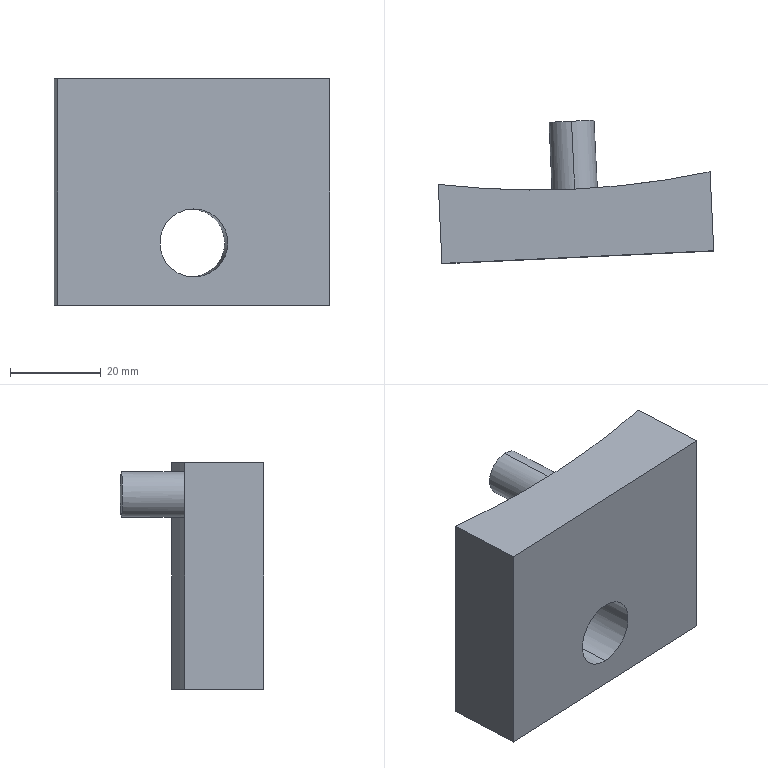Part | SolidWorks | features BaseBody 1 | 1 solid | 11 faces | box 60.748 x 31.599 x 50 mm | volume 45964 mm3 | plane 6 | cylinder 5 | commonest cylinder face diameters 10 x2 15 x2 370 x1
STEP:
#1=CARTESIAN_POINT('',(272.068,803.412,-350.888));
#2=VERTEX_POINT('',#1);
#3=CARTESIAN_POINT('',(272.068,803.412,-365.888));
#4=VERTEX_POINT('',#3);
#5=CARTESIAN_POINT('',(272.068,803.412,-358.388));
#6=DIRECTION('',(-0.04661,0.9989,0.));
#7=DIRECTION('',(0.,0.,1.));
#8=AXIS2_PLACEMENT_3D('',#5,#6,#7);
#9=CIRCLE('',#8,7.5);
#10=EDGE_CURVE('',#2,#4,#9,.T.);
#11=ORIENTED_EDGE('',*,*,#10,.T.);
#12=CARTESIAN_POINT('',(272.068,803.412,-358.388));
#13=DIRECTION('',(-0.04661,0.9989,0.));
#14=DIRECTION('',(0.,0.,1.));
#15=AXIS2_PLACEMENT_3D('',#12,#13,#14);
#16=CIRCLE('',#15,7.5);
#17=EDGE_CURVE('',#4,#2,#16,.T.);
#18=ORIENTED_EDGE('',*,*,#17,.T.);
#19=EDGE_LOOP('',(#11,#18));
#20=FACE_BOUND('',#19,.T.);
#21=CARTESIAN_POINT('',(242.101,802.014,-372.148));
#22=VERTEX_POINT('',#21);
#23=CARTESIAN_POINT('',(302.036,804.81,-372.148));
#24=VERTEX_POINT('',#23);
#25=CARTESIAN_POINT('',(272.068,803.412,-372.148));
#26=DIRECTION('',(0.9989,0.04661,0.));
#27=VECTOR('',#26,1000.);
#28=LINE('',#25,#27);
#29=EDGE_CURVE('',#22,#24,#28,.T.);
#30=ORIENTED_EDGE('',*,*,#29,.T.);
#31=CARTESIAN_POINT('',(302.036,804.81,-322.148));
#32=VERTEX_POINT('',#31);
#33=CARTESIAN_POINT('',(302.036,804.81,-372.148));
#34=DIRECTION('',(0.,0.,-1.));
#35=VECTOR('',#34,1000.);
#36=LINE('',#33,#35);
#37=EDGE_CURVE('',#32,#24,#36,.T.);
#38=ORIENTED_EDGE('',*,*,#37,.F.);
#39=CARTESIAN_POINT('',(242.101,802.014,-322.148));
#40=VERTEX_POINT('',#39);
#41=CARTESIAN_POINT('',(272.068,803.412,-322.148));
#42=DIRECTION('',(0.9989,0.04661,0.));
#43=VECTOR('',#42,1000.);
#44=LINE('',#41,#43);
#45=EDGE_CURVE('',#40,#32,#44,.T.);
#46=ORIENTED_EDGE('',*,*,#45,.F.);
#47=CARTESIAN_POINT('',(242.101,802.014,-372.148));
#48=DIRECTION('',(0.,0.,1.));
#49=VECTOR('',#48,1000.);
#50=LINE('',#47,#49);
#51=EDGE_CURVE('',#22,#40,#50,.T.);
#52=ORIENTED_EDGE('',*,*,#51,.F.);
#53=EDGE_LOOP('',(#30,#38,#46,#52));
#54=FACE_OUTER_BOUND('',#53,.T.);
#55=CARTESIAN_POINT('',(488.568,813.514,-533.369));
#56=DIRECTION('',(-0.04661,0.9989,0.));
#57=DIRECTION('',(0.,0.,1.));
#58=AXIS2_PLACEMENT_3D('',#55,#56,#57);
#59=PLANE('',#58);
#60=ADVANCED_FACE('',(#20,#54),#59,.F.);
#61=CARTESIAN_POINT('',(271.369,818.396,-365.888));
#62=VERTEX_POINT('',#61);
#63=CARTESIAN_POINT('',(272.301,798.417,-365.888));
#64=DIRECTION('',(0.04661,-0.9989,0.));
#65=VECTOR('',#64,1000.);
#66=LINE('',#63,#65);
#67=EDGE_CURVE('',#62,#4,#66,.T.);
#68=ORIENTED_EDGE('',*,*,#67,.T.);
#69=ORIENTED_EDGE('',*,*,#10,.F.);
#70=CARTESIAN_POINT('',(271.369,818.396,-350.888));
#71=VERTEX_POINT('',#70);
#72=CARTESIAN_POINT('',(272.301,798.417,-350.888));
#73=DIRECTION('',(0.04661,-0.9989,0.));
#74=VECTOR('',#73,1000.);
#75=LINE('',#72,#74);
#76=EDGE_CURVE('',#71,#2,#75,.T.);
#77=ORIENTED_EDGE('',*,*,#76,.F.);
#78=CARTESIAN_POINT('',(271.369,818.396,-350.888));
#79=CARTESIAN_POINT('',(271.833,818.417,-350.888));
#80=CARTESIAN_POINT('',(272.31,818.441,-350.931));
#81=CARTESIAN_POINT('',(273.033,818.481,-351.071));
#82=CARTESIAN_POINT('',(273.274,818.494,-351.13));
#83=CARTESIAN_POINT('',(273.636,818.515,-351.239));
#84=CARTESIAN_POINT('',(273.817,818.526,-351.298));
#85=CARTESIAN_POINT('',(274.027,818.539,-351.376));
#86=CARTESIAN_POINT('',(274.132,818.545,-351.417));
#87=CARTESIAN_POINT('',(274.184,818.549,-351.438));
#88=CARTESIAN_POINT('',(274.211,818.55,-351.449));
#89=CARTESIAN_POINT('',(274.222,818.551,-351.453));
#90=CARTESIAN_POINT('',(274.229,818.551,-351.456));
#91=CARTESIAN_POINT('',(274.234,818.552,-351.458));
#92=CARTESIAN_POINT('',(274.545,818.571,-351.587));
#93=CARTESIAN_POINT('',(274.918,818.595,-351.765));
#94=CARTESIAN_POINT('',(275.749,818.652,-352.285));
#95=CARTESIAN_POINT('',(276.207,818.684,-352.627));
#96=CARTESIAN_POINT('',(277.12,818.753,-353.542));
#97=CARTESIAN_POINT('',(277.461,818.78,-354.002));
#98=CARTESIAN_POINT('',(277.85,818.812,-354.626));
#99=CARTESIAN_POINT('',(277.959,818.821,-354.823));
#100=CARTESIAN_POINT('',(278.098,818.832,-355.099));
#101=CARTESIAN_POINT('',(278.14,818.836,-355.188));
#102=CARTESIAN_POINT('',(278.198,818.841,-355.315));
#103=CARTESIAN_POINT('',(278.225,818.843,-355.377));
#104=CARTESIAN_POINT('',(278.255,818.846,-355.447));
#105=CARTESIAN_POINT('',(278.27,818.847,-355.481));
#106=CARTESIAN_POINT('',(278.277,818.848,-355.499));
#107=CARTESIAN_POINT('',(278.28,818.848,-355.506));
#108=CARTESIAN_POINT('',(278.282,818.848,-355.511));
#109=CARTESIAN_POINT('',(278.282,818.848,-355.512));
#110=CARTESIAN_POINT('',(278.481,818.865,-355.993));
#111=CARTESIAN_POINT('',(278.624,818.877,-356.479));
#112=CARTESIAN_POINT('',(278.81,818.893,-357.442));
#113=CARTESIAN_POINT('',(278.854,818.897,-357.919));
#114=CARTESIAN_POINT('',(278.854,818.897,-358.847));
#115=CARTESIAN_POINT('',(278.812,818.893,-359.324));
#116=CARTESIAN_POINT('',(278.673,818.881,-360.047));
#117=CARTESIAN_POINT('',(278.614,818.876,-360.289));
#118=CARTESIAN_POINT('',(278.507,818.867,-360.651));
#119=CARTESIAN_POINT('',(278.448,818.862,-360.832));
#120=CARTESIAN_POINT('',(278.37,818.856,-361.043));
#121=CARTESIAN_POINT('',(278.33,818.852,-361.148));
#122=CARTESIAN_POINT('',(278.309,818.85,-361.2));
#123=CARTESIAN_POINT('',(278.298,818.849,-361.226));
#124=CARTESIAN_POINT('',(278.293,818.849,-361.237));
#125=CARTESIAN_POINT('',(278.29,818.849,-361.245));
#126=CARTESIAN_POINT('',(278.288,818.849,-361.25));
#127=CARTESIAN_POINT('',(278.16,818.838,-361.562));
#128=CARTESIAN_POINT('',(277.983,818.823,-361.936));
#129=CARTESIAN_POINT('',(277.465,818.781,-362.77));
#130=CARTESIAN_POINT('',(277.124,818.754,-363.229));
#131=CARTESIAN_POINT('',(276.21,818.685,-364.146));
#132=CARTESIAN_POINT('',(275.751,818.652,-364.489));
#133=CARTESIAN_POINT('',(275.128,818.61,-364.88));
#134=CARTESIAN_POINT('',(274.93,818.596,-364.989));
#135=CARTESIAN_POINT('',(274.655,818.578,-365.128));
#136=CARTESIAN_POINT('',(274.566,818.573,-365.171));
#137=CARTESIAN_POINT('',(274.439,818.565,-365.229));
#138=CARTESIAN_POINT('',(274.377,818.561,-365.257));
#139=CARTESIAN_POINT('',(274.307,818.556,-365.287));
#140=CARTESIAN_POINT('',(274.273,818.554,-365.301));
#141=CARTESIAN_POINT('',(274.256,818.553,-365.309));
#142=CARTESIAN_POINT('',(274.249,818.553,-365.312));
#143=CARTESIAN_POINT('',(274.244,818.552,-365.314));
#144=CARTESIAN_POINT('',(274.243,818.552,-365.314));
#145=CARTESIAN_POINT('',(273.283,818.492,-365.713));
#146=CARTESIAN_POINT('',(272.297,818.439,-365.888));
#147=CARTESIAN_POINT('',(271.369,818.396,-365.888));
#148=B_SPLINE_CURVE_WITH_KNOTS('',3,(#78,#79,#80,#81,#82,#83,#84,#85,#86,#87,#88,#89,#90,#91,#92,#93,#94,#95,#96,#97,#98,#99,#100,#101,#102,#103,#104,#105,#106,#107,#108,#109,#110,#111,#112,#113,#114,#115,#116,#117,#118,#119,#120,#121,#122,#123,#124,#125,#126,#127,#128,#129,#130,#131,#132,#133,#134,#135,#136,#137,#138,#139,#140,#141,#142,#143,#144,#145,#146,#147),.UNSPECIFIED.,.F.,.F.,(4,2,2,1,1,1,1,1,2,2,2,2,2,2,2,1,1,1,1,2,2,2,2,2,2,1,1,1,1,1,2,2,2,2,2,2,2,1,1,1,1,2,2,4),(0.,0.0625,0.09375,0.1094,0.1172,0.1211,0.123,0.124,0.1245,0.125,0.1875,0.25,0.3125,0.3438,0.3594,0.3672,0.3711,0.373,0.374,0.3745,0.375,0.4375,0.5,0.5625,0.5937,0.6094,0.6172,0.6211,0.623,0.624,0.6245,0.625,0.6875,0.75,0.8125,0.8437,0.8594,0.8672,0.8711,0.873,0.874,0.8745,0.875,1.),.UNSPECIFIED.);
#149=EDGE_CURVE('',#71,#62,#148,.T.);
#150=ORIENTED_EDGE('',*,*,#149,.T.);
#151=EDGE_LOOP('',(#68,#69,#77,#150));
#152=FACE_OUTER_BOUND('',#151,.T.);
#153=CARTESIAN_POINT('',(272.301,798.417,-358.388));
#154=DIRECTION('',(-0.04661,0.9989,0.));
#155=DIRECTION('',(0.,0.,-1.));
#156=AXIS2_PLACEMENT_3D('',#153,#154,#155);
#157=CYLINDRICAL_SURFACE('',#156,7.5);
#158=ADVANCED_FACE('',(#152),#157,.F.);
#159=CARTESIAN_POINT('',(270.67,833.379,-324.148));
#160=VERTEX_POINT('',#159);
#161=CARTESIAN_POINT('',(270.67,833.379,-334.148));
#162=VERTEX_POINT('',#161);
#163=CARTESIAN_POINT('',(270.67,833.379,-329.148));
#164=DIRECTION('',(0.04661,-0.9989,0.));
#165=DIRECTION('',(0.,0.,-1.));
#166=AXIS2_PLACEMENT_3D('',#163,#164,#165);
#167=CIRCLE('',#166,5.);
#168=EDGE_CURVE('',#160,#162,#167,.T.);
#169=ORIENTED_EDGE('',*,*,#168,.F.);
#170=CARTESIAN_POINT('',(270.67,833.379,-329.148));
#171=DIRECTION('',(0.04661,-0.9989,0.));
#172=DIRECTION('',(0.,0.,-1.));
#173=AXIS2_PLACEMENT_3D('',#170,#171,#172);
#174=CIRCLE('',#173,5.);
#175=EDGE_CURVE('',#162,#160,#174,.T.);
#176=ORIENTED_EDGE('',*,*,#175,.F.);
#177=EDGE_LOOP('',(#169,#176));
#178=FACE_OUTER_BOUND('',#177,.T.);
#179=CARTESIAN_POINT('',(270.67,833.379,-329.148));
#180=DIRECTION('',(0.04661,-0.9989,0.));
#181=DIRECTION('',(0.,0.,-1.));
#182=AXIS2_PLACEMENT_3D('',#179,#180,#181);
#183=PLANE('',#182);
#184=ADVANCED_FACE('',(#178),#183,.F.);
#185=CARTESIAN_POINT('',(271.369,818.396,-334.148));
#186=VERTEX_POINT('',#185);
#187=CARTESIAN_POINT('',(272.302,798.416,-334.148));
#188=DIRECTION('',(0.04661,-0.9989,0.));
#189=VECTOR('',#188,1000.);
#190=LINE('',#187,#189);
#191=EDGE_CURVE('',#162,#186,#190,.T.);
#192=ORIENTED_EDGE('',*,*,#191,.T.);
#193=CARTESIAN_POINT('',(271.369,818.396,-324.148));
#194=VERTEX_POINT('',#193);
#195=CARTESIAN_POINT('',(271.369,818.396,-334.148));
#196=CARTESIAN_POINT('',(271.06,818.381,-334.148));
#197=CARTESIAN_POINT('',(270.742,818.367,-334.119));
#198=CARTESIAN_POINT('',(270.26,818.347,-334.026));
#199=CARTESIAN_POINT('',(270.099,818.341,-333.986));
#200=CARTESIAN_POINT('',(269.857,818.331,-333.914));
#201=CARTESIAN_POINT('',(269.737,818.327,-333.875));
#202=CARTESIAN_POINT('',(269.596,818.321,-333.823));
#203=CARTESIAN_POINT('',(269.526,818.319,-333.795));
#204=CARTESIAN_POINT('',(269.491,818.318,-333.781));
#205=CARTESIAN_POINT('',(269.477,818.317,-333.775));
#206=CARTESIAN_POINT('',(269.467,818.317,-333.771));
#207=CARTESIAN_POINT('',(269.46,818.316,-333.768));
#208=CARTESIAN_POINT('',(269.251,818.309,-333.682));
#209=CARTESIAN_POINT('',(269.002,818.3,-333.563));
#210=CARTESIAN_POINT('',(268.447,818.282,-333.217));
#211=CARTESIAN_POINT('',(268.141,818.273,-332.989));
#212=CARTESIAN_POINT('',(267.531,818.256,-332.378));
#213=CARTESIAN_POINT('',(267.303,818.25,-332.072));
#214=CARTESIAN_POINT('',(267.043,818.244,-331.656));
#215=CARTESIAN_POINT('',(266.97,818.243,-331.524));
#216=CARTESIAN_POINT('',(266.877,818.241,-331.34));
#217=CARTESIAN_POINT('',(266.849,818.24,-331.281));
#218=CARTESIAN_POINT('',(266.81,818.239,-331.197));
#219=CARTESIAN_POINT('',(266.792,818.239,-331.155));
#220=CARTESIAN_POINT('',(266.772,818.238,-331.108));
#221=CARTESIAN_POINT('',(266.762,818.238,-331.086));
#222=CARTESIAN_POINT('',(266.758,818.238,-331.076));
#223=CARTESIAN_POINT('',(266.756,818.238,-331.069));
#224=CARTESIAN_POINT('',(266.755,818.238,-331.068));
#225=CARTESIAN_POINT('',(266.489,818.232,-330.426));
#226=CARTESIAN_POINT('',(266.372,818.23,-329.77));
#227=CARTESIAN_POINT('',(266.371,818.23,-328.842));
#228=CARTESIAN_POINT('',(266.4,818.231,-328.524));
#229=CARTESIAN_POINT('',(266.493,818.232,-328.042));
#230=CARTESIAN_POINT('',(266.532,818.233,-327.881));
#231=CARTESIAN_POINT('',(266.604,818.235,-327.639));
#232=CARTESIAN_POINT('',(266.643,818.236,-327.519));
#233=CARTESIAN_POINT('',(266.695,818.237,-327.378));
#234=CARTESIAN_POINT('',(266.722,818.237,-327.308));
#235=CARTESIAN_POINT('',(266.736,818.238,-327.273));
#236=CARTESIAN_POINT('',(266.742,818.238,-327.258));
#237=CARTESIAN_POINT('',(266.746,818.238,-327.248));
#238=CARTESIAN_POINT('',(266.749,818.238,-327.242));
#239=CARTESIAN_POINT('',(266.836,818.24,-327.032));
#240=CARTESIAN_POINT('',(266.954,818.242,-326.783));
#241=CARTESIAN_POINT('',(267.3,818.25,-326.227));
#242=CARTESIAN_POINT('',(267.528,818.256,-325.921));
#243=CARTESIAN_POINT('',(268.139,818.273,-325.309));
#244=CARTESIAN_POINT('',(268.445,818.282,-325.08));
#245=CARTESIAN_POINT('',(268.862,818.296,-324.82));
#246=CARTESIAN_POINT('',(268.994,818.3,-324.747));
#247=CARTESIAN_POINT('',(269.178,818.306,-324.654));
#248=CARTESIAN_POINT('',(269.237,818.309,-324.626));
#249=CARTESIAN_POINT('',(269.321,818.311,-324.587));
#250=CARTESIAN_POINT('',(269.363,818.313,-324.569));
#251=CARTESIAN_POINT('',(269.41,818.315,-324.549));
#252=CARTESIAN_POINT('',(269.432,818.315,-324.539));
#253=CARTESIAN_POINT('',(269.442,818.316,-324.535));
#254=CARTESIAN_POINT('',(269.449,818.316,-324.532));
#255=CARTESIAN_POINT('',(269.45,818.316,-324.532));
#256=CARTESIAN_POINT('',(270.093,818.339,-324.265));
#257=CARTESIAN_POINT('',(270.751,818.367,-324.148));
#258=CARTESIAN_POINT('',(271.369,818.396,-324.148));
#259=B_SPLINE_CURVE_WITH_KNOTS('',3,(#195,#196,#197,#198,#199,#200,#201,#202,#203,#204,#205,#206,#207,#208,#209,#210,#211,#212,#213,#214,#215,#216,#217,#218,#219,#220,#221,#222,#223,#224,#225,#226,#227,#228,#229,#230,#231,#232,#233,#234,#235,#236,#237,#238,#239,#240,#241,#242,#243,#244,#245,#246,#247,#248,#249,#250,#251,#252,#253,#254,#255,#256,#257,#258),.UNSPECIFIED.,.F.,.F.,(4,2,2,1,1,1,1,2,2,2,2,2,2,2,1,1,1,2,2,2,2,2,1,1,1,1,2,2,2,2,2,2,2,1,1,1,2,2,4),(0.,0.0625,0.09375,0.1094,0.1172,0.1211,0.123,0.124,0.125,0.1875,0.25,0.3125,0.3438,0.3594,0.3672,0.3711,0.373,0.374,0.375,0.5,0.5625,0.5938,0.6094,0.6172,0.6211,0.623,0.624,0.625,0.6875,0.75,0.8125,0.8438,0.8594,0.8672,0.8711,0.873,0.874,0.875,1.),.UNSPECIFIED.);
#260=EDGE_CURVE('',#186,#194,#259,.T.);
#261=ORIENTED_EDGE('',*,*,#260,.T.);
#262=CARTESIAN_POINT('',(272.302,798.416,-324.148));
#263=DIRECTION('',(0.04661,-0.9989,0.));
#264=VECTOR('',#263,1000.);
#265=LINE('',#262,#264);
#266=EDGE_CURVE('',#160,#194,#265,.T.);
#267=ORIENTED_EDGE('',*,*,#266,.F.);
#268=ORIENTED_EDGE('',*,*,#168,.T.);
#269=EDGE_LOOP('',(#192,#261,#267,#268));
#270=FACE_OUTER_BOUND('',#269,.T.);
#271=CARTESIAN_POINT('',(272.302,798.416,-329.148));
#272=DIRECTION('',(-0.04661,0.9989,0.));
#273=DIRECTION('',(0.,0.,-1.));
#274=AXIS2_PLACEMENT_3D('',#271,#272,#273);
#275=CYLINDRICAL_SURFACE('',#274,5.);
#276=ADVANCED_FACE('',(#270),#275,.T.);
#277=CARTESIAN_POINT('',(241.288,819.443,-322.148));
#278=VERTEX_POINT('',#277);
#279=CARTESIAN_POINT('',(241.288,819.443,-322.148));
#280=DIRECTION('',(-0.04661,0.9989,0.));
#281=VECTOR('',#280,1000.);
#282=LINE('',#279,#281);
#283=EDGE_CURVE('',#40,#278,#282,.T.);
#284=ORIENTED_EDGE('',*,*,#283,.F.);
#285=ORIENTED_EDGE('',*,*,#45,.T.);
#286=CARTESIAN_POINT('',(301.223,822.24,-322.148));
#287=VERTEX_POINT('',#286);
#288=CARTESIAN_POINT('',(301.223,822.24,-322.148));
#289=DIRECTION('',(0.04661,-0.9989,0.));
#290=VECTOR('',#289,1000.);
#291=LINE('',#288,#290);
#292=EDGE_CURVE('',#287,#32,#291,.T.);
#293=ORIENTED_EDGE('',*,*,#292,.F.);
#294=CARTESIAN_POINT('',(262.746,1003.195,-322.148));
#295=DIRECTION('',(0.,0.,1.));
#296=DIRECTION('',(0.9989,0.04661,0.));
#297=AXIS2_PLACEMENT_3D('',#294,#295,#296);
#298=CIRCLE('',#297,185.);
#299=EDGE_CURVE('',#278,#287,#298,.T.);
#300=ORIENTED_EDGE('',*,*,#299,.F.);
#301=EDGE_LOOP('',(#284,#285,#293,#300));
#302=FACE_OUTER_BOUND('',#301,.T.);
#303=CARTESIAN_POINT('',(262.746,1003.195,-322.148));
#304=DIRECTION('',(0.,0.,-1.));
#305=DIRECTION('',(0.,-1.,0.));
#306=AXIS2_PLACEMENT_3D('',#303,#304,#305);
#307=PLANE('',#306);
#308=ADVANCED_FACE('',(#302),#307,.F.);
#309=ORIENTED_EDGE('',*,*,#29,.F.);
#310=CARTESIAN_POINT('',(241.288,819.443,-372.148));
#311=VERTEX_POINT('',#310);
#312=CARTESIAN_POINT('',(241.288,819.443,-372.148));
#313=DIRECTION('',(-0.04661,0.9989,0.));
#314=VECTOR('',#313,1000.);
#315=LINE('',#312,#314);
#316=EDGE_CURVE('',#22,#311,#315,.T.);
#317=ORIENTED_EDGE('',*,*,#316,.T.);
#318=CARTESIAN_POINT('',(301.223,822.24,-372.148));
#319=VERTEX_POINT('',#318);
#320=CARTESIAN_POINT('',(262.746,1003.195,-372.148));
#321=DIRECTION('',(0.,0.,1.));
#322=DIRECTION('',(0.9989,0.04661,0.));
#323=AXIS2_PLACEMENT_3D('',#320,#321,#322);
#324=CIRCLE('',#323,185.);
#325=EDGE_CURVE('',#311,#319,#324,.T.);
#326=ORIENTED_EDGE('',*,*,#325,.T.);
#327=CARTESIAN_POINT('',(301.223,822.24,-372.148));
#328=DIRECTION('',(0.04661,-0.9989,0.));
#329=VECTOR('',#328,1000.);
#330=LINE('',#327,#329);
#331=EDGE_CURVE('',#319,#24,#330,.T.);
#332=ORIENTED_EDGE('',*,*,#331,.T.);
#333=EDGE_LOOP('',(#309,#317,#326,#332));
#334=FACE_OUTER_BOUND('',#333,.T.);
#335=CARTESIAN_POINT('',(262.746,1003.195,-372.148));
#336=DIRECTION('',(0.,0.,-1.));
#337=DIRECTION('',(0.,-1.,0.));
#338=AXIS2_PLACEMENT_3D('',#335,#336,#337);
#339=PLANE('',#338);
#340=ADVANCED_FACE('',(#334),#339,.T.);
#341=ORIENTED_EDGE('',*,*,#316,.F.);
#342=ORIENTED_EDGE('',*,*,#51,.T.);
#343=ORIENTED_EDGE('',*,*,#283,.T.);
#344=CARTESIAN_POINT('',(241.288,819.443,-372.148));
#345=DIRECTION('',(0.,0.,1.));
#346=VECTOR('',#345,1000.);
#347=LINE('',#344,#346);
#348=EDGE_CURVE('',#311,#278,#347,.T.);
#349=ORIENTED_EDGE('',*,*,#348,.F.);
#350=EDGE_LOOP('',(#341,#342,#343,#349));
#351=FACE_OUTER_BOUND('',#350,.T.);
#352=CARTESIAN_POINT('',(241.288,819.443,-372.148));
#353=DIRECTION('',(0.9989,0.04661,0.));
#354=DIRECTION('',(0.,0.,-1.));
#355=AXIS2_PLACEMENT_3D('',#352,#353,#354);
#356=PLANE('',#355);
#357=ADVANCED_FACE('',(#351),#356,.F.);
#358=ORIENTED_EDGE('',*,*,#292,.T.);
#359=ORIENTED_EDGE('',*,*,#37,.T.);
#360=ORIENTED_EDGE('',*,*,#331,.F.);
#361=CARTESIAN_POINT('',(301.223,822.24,-372.148));
#362=DIRECTION('',(0.,0.,1.));
#363=VECTOR('',#362,1000.);
#364=LINE('',#361,#363);
#365=EDGE_CURVE('',#319,#287,#364,.T.);
#366=ORIENTED_EDGE('',*,*,#365,.T.);
#367=EDGE_LOOP('',(#358,#359,#360,#366));
#368=FACE_OUTER_BOUND('',#367,.T.);
#369=CARTESIAN_POINT('',(301.223,822.24,-372.148));
#370=DIRECTION('',(-0.9989,-0.04661,0.));
#371=DIRECTION('',(-0.04661,0.9989,0.));
#372=AXIS2_PLACEMENT_3D('',#369,#370,#371);
#373=PLANE('',#372);
#374=ADVANCED_FACE('',(#368),#373,.F.);
#375=ORIENTED_EDGE('',*,*,#149,.F.);
#376=CARTESIAN_POINT('',(271.369,818.396,-365.888));
#377=CARTESIAN_POINT('',(270.906,818.374,-365.888));
#378=CARTESIAN_POINT('',(270.428,818.354,-365.845));
#379=CARTESIAN_POINT('',(269.705,818.325,-365.705));
#380=CARTESIAN_POINT('',(269.463,818.317,-365.646));
#381=CARTESIAN_POINT('',(269.101,818.304,-365.537));
#382=CARTESIAN_POINT('',(268.92,818.298,-365.478));
#383=CARTESIAN_POINT('',(268.71,818.291,-365.4));
#384=CARTESIAN_POINT('',(268.605,818.287,-365.359));
#385=CARTESIAN_POINT('',(268.552,818.286,-365.338));
#386=CARTESIAN_POINT('',(268.526,818.285,-365.327));
#387=CARTESIAN_POINT('',(268.515,818.285,-365.323));
#388=CARTESIAN_POINT('',(268.507,818.284,-365.32));
#389=CARTESIAN_POINT('',(268.502,818.284,-365.317));
#390=CARTESIAN_POINT('',(268.191,818.274,-365.189));
#391=CARTESIAN_POINT('',(267.818,818.264,-365.011));
#392=CARTESIAN_POINT('',(266.985,818.243,-364.491));
#393=CARTESIAN_POINT('',(266.526,818.233,-364.149));
#394=CARTESIAN_POINT('',(265.61,818.216,-363.234));
#395=CARTESIAN_POINT('',(265.268,818.211,-362.774));
#396=CARTESIAN_POINT('',(264.878,818.207,-362.15));
#397=CARTESIAN_POINT('',(264.769,818.205,-361.953));
#398=CARTESIAN_POINT('',(264.63,818.204,-361.677));
#399=CARTESIAN_POINT('',(264.587,818.204,-361.588));
#400=CARTESIAN_POINT('',(264.529,818.203,-361.461));
#401=CARTESIAN_POINT('',(264.501,818.203,-361.399));
#402=CARTESIAN_POINT('',(264.471,818.203,-361.329));
#403=CARTESIAN_POINT('',(264.457,818.203,-361.294));
#404=CARTESIAN_POINT('',(264.45,818.202,-361.277));
#405=CARTESIAN_POINT('',(264.447,818.202,-361.27));
#406=CARTESIAN_POINT('',(264.445,818.202,-361.265));
#407=CARTESIAN_POINT('',(264.444,818.202,-361.264));
#408=CARTESIAN_POINT('',(264.244,818.201,-360.783));
#409=CARTESIAN_POINT('',(264.101,818.199,-360.297));
#410=CARTESIAN_POINT('',(263.914,818.198,-359.334));
#411=CARTESIAN_POINT('',(263.871,818.198,-358.857));
#412=CARTESIAN_POINT('',(263.87,818.198,-357.929));
#413=CARTESIAN_POINT('',(263.913,818.198,-357.452));
#414=CARTESIAN_POINT('',(264.052,818.199,-356.729));
#415=CARTESIAN_POINT('',(264.111,818.2,-356.487));
#416=CARTESIAN_POINT('',(264.219,818.2,-356.125));
#417=CARTESIAN_POINT('',(264.278,818.201,-355.944));
#418=CARTESIAN_POINT('',(264.356,818.202,-355.733));
#419=CARTESIAN_POINT('',(264.397,818.202,-355.628));
#420=CARTESIAN_POINT('',(264.418,818.202,-355.576));
#421=CARTESIAN_POINT('',(264.428,818.202,-355.55));
#422=CARTESIAN_POINT('',(264.433,818.202,-355.539));
#423=CARTESIAN_POINT('',(264.436,818.202,-355.531));
#424=CARTESIAN_POINT('',(264.438,818.202,-355.526));
#425=CARTESIAN_POINT('',(264.567,818.204,-355.214));
#426=CARTESIAN_POINT('',(264.745,818.205,-354.84));
#427=CARTESIAN_POINT('',(265.264,818.211,-354.006));
#428=CARTESIAN_POINT('',(265.606,818.216,-353.547));
#429=CARTESIAN_POINT('',(266.523,818.233,-352.63));
#430=CARTESIAN_POINT('',(266.982,818.243,-352.287));
#431=CARTESIAN_POINT('',(267.607,818.259,-351.896));
#432=CARTESIAN_POINT('',(267.805,818.264,-351.787));
#433=CARTESIAN_POINT('',(268.081,818.272,-351.647));
#434=CARTESIAN_POINT('',(268.17,818.274,-351.605));
#435=CARTESIAN_POINT('',(268.297,818.278,-351.547));
#436=CARTESIAN_POINT('',(268.359,818.28,-351.519));
#437=CARTESIAN_POINT('',(268.429,818.282,-351.489));
#438=CARTESIAN_POINT('',(268.464,818.283,-351.475));
#439=CARTESIAN_POINT('',(268.481,818.283,-351.467));
#440=CARTESIAN_POINT('',(268.488,818.284,-351.464));
#441=CARTESIAN_POINT('',(268.493,818.284,-351.462));
#442=CARTESIAN_POINT('',(268.494,818.284,-351.462));
#443=CARTESIAN_POINT('',(269.455,818.314,-351.063));
#444=CARTESIAN_POINT('',(270.441,818.352,-350.888));
#445=CARTESIAN_POINT('',(271.369,818.396,-350.888));
#446=B_SPLINE_CURVE_WITH_KNOTS('',3,(#376,#377,#378,#379,#380,#381,#382,#383,#384,#385,#386,#387,#388,#389,#390,#391,#392,#393,#394,#395,#396,#397,#398,#399,#400,#401,#402,#403,#404,#405,#406,#407,#408,#409,#410,#411,#412,#413,#414,#415,#416,#417,#418,#419,#420,#421,#422,#423,#424,#425,#426,#427,#428,#429,#430,#431,#432,#433,#434,#435,#436,#437,#438,#439,#440,#441,#442,#443,#444,#445),.UNSPECIFIED.,.F.,.F.,(4,2,2,1,1,1,1,1,2,2,2,2,2,2,2,1,1,1,1,2,2,2,2,2,2,1,1,1,1,1,2,2,2,2,2,2,2,1,1,1,1,2,2,4),(0.,0.0625,0.09375,0.1094,0.1172,0.1211,0.123,0.124,0.1245,0.125,0.1875,0.25,0.3125,0.3437,0.3594,0.3672,0.3711,0.373,0.374,0.3745,0.375,0.4375,0.5,0.5625,0.5938,0.6094,0.6172,0.6211,0.623,0.624,0.6245,0.625,0.6875,0.75,0.8125,0.8438,0.8594,0.8672,0.8711,0.873,0.874,0.8745,0.875,1.),.UNSPECIFIED.);
#447=EDGE_CURVE('',#62,#71,#446,.T.);
#448=ORIENTED_EDGE('',*,*,#447,.F.);
#449=EDGE_LOOP('',(#375,#448));
#450=FACE_BOUND('',#449,.T.);
#451=CARTESIAN_POINT('',(271.369,818.396,-324.148));
#452=CARTESIAN_POINT('',(271.678,818.41,-324.148));
#453=CARTESIAN_POINT('',(271.997,818.426,-324.177));
#454=CARTESIAN_POINT('',(272.478,818.451,-324.27));
#455=CARTESIAN_POINT('',(272.639,818.459,-324.309));
#456=CARTESIAN_POINT('',(272.881,818.472,-324.382));
#457=CARTESIAN_POINT('',(273.001,818.479,-324.421));
#458=CARTESIAN_POINT('',(273.141,818.487,-324.473));
#459=CARTESIAN_POINT('',(273.211,818.491,-324.501));
#460=CARTESIAN_POINT('',(273.246,818.493,-324.515));
#461=CARTESIAN_POINT('',(273.261,818.494,-324.521));
#462=CARTESIAN_POINT('',(273.271,818.494,-324.525));
#463=CARTESIAN_POINT('',(273.278,818.495,-324.528));
#464=CARTESIAN_POINT('',(273.486,818.507,-324.614));
#465=CARTESIAN_POINT('',(273.735,818.521,-324.733));
#466=CARTESIAN_POINT('',(274.289,818.555,-325.079));
#467=CARTESIAN_POINT('',(274.595,818.574,-325.307));
#468=CARTESIAN_POINT('',(275.204,818.614,-325.918));
#469=CARTESIAN_POINT('',(275.432,818.63,-326.224));
#470=CARTESIAN_POINT('',(275.691,818.648,-326.64));
#471=CARTESIAN_POINT('',(275.763,818.653,-326.772));
#472=CARTESIAN_POINT('',(275.856,818.66,-326.955));
#473=CARTESIAN_POINT('',(275.884,818.662,-327.014));
#474=CARTESIAN_POINT('',(275.923,818.664,-327.099));
#475=CARTESIAN_POINT('',(275.941,818.666,-327.141));
#476=CARTESIAN_POINT('',(275.961,818.667,-327.187));
#477=CARTESIAN_POINT('',(275.971,818.668,-327.21));
#478=CARTESIAN_POINT('',(275.975,818.668,-327.22));
#479=CARTESIAN_POINT('',(275.978,818.668,-327.227));
#480=CARTESIAN_POINT('',(275.978,818.668,-327.228));
#481=CARTESIAN_POINT('',(276.244,818.687,-327.87));
#482=CARTESIAN_POINT('',(276.36,818.696,-328.526));
#483=CARTESIAN_POINT('',(276.361,818.696,-329.454));
#484=CARTESIAN_POINT('',(276.332,818.694,-329.772));
#485=CARTESIAN_POINT('',(276.24,818.687,-330.254));
#486=CARTESIAN_POINT('',(276.201,818.684,-330.415));
#487=CARTESIAN_POINT('',(276.129,818.679,-330.657));
#488=CARTESIAN_POINT('',(276.09,818.676,-330.777));
#489=CARTESIAN_POINT('',(276.038,818.673,-330.918));
#490=CARTESIAN_POINT('',(276.011,818.671,-330.988));
#491=CARTESIAN_POINT('',(275.997,818.67,-331.023));
#492=CARTESIAN_POINT('',(275.991,818.669,-331.038));
#493=CARTESIAN_POINT('',(275.987,818.669,-331.047));
#494=CARTESIAN_POINT('',(275.984,818.669,-331.054));
#495=CARTESIAN_POINT('',(275.898,818.663,-331.264));
#496=CARTESIAN_POINT('',(275.779,818.654,-331.513));
#497=CARTESIAN_POINT('',(275.434,818.63,-332.069));
#498=CARTESIAN_POINT('',(275.207,818.614,-332.375));
#499=CARTESIAN_POINT('',(274.597,818.574,-332.987));
#500=CARTESIAN_POINT('',(274.291,818.555,-333.216));
#501=CARTESIAN_POINT('',(273.875,818.53,-333.476));
#502=CARTESIAN_POINT('',(273.743,818.522,-333.549));
#503=CARTESIAN_POINT('',(273.56,818.511,-333.642));
#504=CARTESIAN_POINT('',(273.501,818.507,-333.67));
#505=CARTESIAN_POINT('',(273.416,818.503,-333.709));
#506=CARTESIAN_POINT('',(273.375,818.5,-333.727));
#507=CARTESIAN_POINT('',(273.328,818.497,-333.747));
#508=CARTESIAN_POINT('',(273.305,818.496,-333.757));
#509=CARTESIAN_POINT('',(273.295,818.496,-333.761));
#510=CARTESIAN_POINT('',(273.289,818.495,-333.764));
#511=CARTESIAN_POINT('',(273.288,818.495,-333.764));
#512=CARTESIAN_POINT('',(272.645,818.459,-334.031));
#513=CARTESIAN_POINT('',(271.988,818.425,-334.148));
#514=CARTESIAN_POINT('',(271.369,818.396,-334.148));
#515=B_SPLINE_CURVE_WITH_KNOTS('',3,(#451,#452,#453,#454,#455,#456,#457,#458,#459,#460,#461,#462,#463,#464,#465,#466,#467,#468,#469,#470,#471,#472,#473,#474,#475,#476,#477,#478,#479,#480,#481,#482,#483,#484,#485,#486,#487,#488,#489,#490,#491,#492,#493,#494,#495,#496,#497,#498,#499,#500,#501,#502,#503,#504,#505,#506,#507,#508,#509,#510,#511,#512,#513,#514),.UNSPECIFIED.,.F.,.F.,(4,2,2,1,1,1,1,2,2,2,2,2,2,2,1,1,1,2,2,2,2,2,1,1,1,1,2,2,2,2,2,2,2,1,1,1,2,2,4),(0.,0.0625,0.09375,0.1094,0.1172,0.1211,0.123,0.124,0.125,0.1875,0.25,0.3125,0.3438,0.3594,0.3672,0.3711,0.373,0.374,0.375,0.5,0.5625,0.5938,0.6094,0.6172,0.6211,0.623,0.624,0.625,0.6875,0.75,0.8125,0.8438,0.8594,0.8672,0.8711,0.873,0.874,0.875,1.),.UNSPECIFIED.);
#516=EDGE_CURVE('',#194,#186,#515,.T.);
#517=ORIENTED_EDGE('',*,*,#516,.F.);
#518=ORIENTED_EDGE('',*,*,#260,.F.);
#519=EDGE_LOOP('',(#517,#518));
#520=FACE_BOUND('',#519,.T.);
#521=ORIENTED_EDGE('',*,*,#299,.T.);
#522=ORIENTED_EDGE('',*,*,#365,.F.);
#523=ORIENTED_EDGE('',*,*,#325,.F.);
#524=ORIENTED_EDGE('',*,*,#348,.T.);
#525=EDGE_LOOP('',(#521,#522,#523,#524));
#526=FACE_OUTER_BOUND('',#525,.T.);
#527=CARTESIAN_POINT('',(262.746,1003.195,-372.148));
#528=DIRECTION('',(0.,0.,1.));
#529=DIRECTION('',(0.9989,0.04661,0.));
#530=AXIS2_PLACEMENT_3D('',#527,#528,#529);
#531=CYLINDRICAL_SURFACE('',#530,185.);
#532=ADVANCED_FACE('',(#450,#520,#526),#531,.F.);
#533=ORIENTED_EDGE('',*,*,#516,.T.);
#534=ORIENTED_EDGE('',*,*,#191,.F.);
#535=ORIENTED_EDGE('',*,*,#175,.T.);
#536=ORIENTED_EDGE('',*,*,#266,.T.);
#537=EDGE_LOOP('',(#533,#534,#535,#536));
#538=FACE_OUTER_BOUND('',#537,.T.);
#539=CARTESIAN_POINT('',(272.302,798.416,-329.148));
#540=DIRECTION('',(-0.04661,0.9989,0.));
#541=DIRECTION('',(0.,0.,-1.));
#542=AXIS2_PLACEMENT_3D('',#539,#540,#541);
#543=CYLINDRICAL_SURFACE('',#542,5.);
#544=ADVANCED_FACE('',(#538),#543,.T.);
#545=ORIENTED_EDGE('',*,*,#17,.F.);
#546=ORIENTED_EDGE('',*,*,#67,.F.);
#547=ORIENTED_EDGE('',*,*,#447,.T.);
#548=ORIENTED_EDGE('',*,*,#76,.T.);
#549=EDGE_LOOP('',(#545,#546,#547,#548));
#550=FACE_OUTER_BOUND('',#549,.T.);
#551=CARTESIAN_POINT('',(272.301,798.417,-358.388));
#552=DIRECTION('',(-0.04661,0.9989,0.));
#553=DIRECTION('',(0.,0.,-1.));
#554=AXIS2_PLACEMENT_3D('',#551,#552,#553);
#555=CYLINDRICAL_SURFACE('',#554,7.5);
#556=ADVANCED_FACE('',(#550),#555,.F.);
#557=CLOSED_SHELL('',(#60,#158,#184,#276,#308,#340,#357,#374,#532,#544,#556));
#558=MANIFOLD_SOLID_BREP('',#557);
#559=CARTESIAN_POINT('',(0.,0.,0.));
#560=DIRECTION('',(0.,0.,1.));
#561=DIRECTION('',(1.,0.,0.));
#562=AXIS2_PLACEMENT_3D('',#559,#560,#561);
#563=(LENGTH_UNIT()NAMED_UNIT(*)SI_UNIT(.MILLI.,.METRE.));
#564=UNCERTAINTY_MEASURE_WITH_UNIT(LENGTH_MEASURE(0.00001),#563,'','');
#565=(NAMED_UNIT(*)PLANE_ANGLE_UNIT()SI_UNIT($,.RADIAN.));
#566=(NAMED_UNIT(*)SI_UNIT($,.STERADIAN.)SOLID_ANGLE_UNIT());
#567=(GEOMETRIC_REPRESENTATION_CONTEXT(3)GLOBAL_UNCERTAINTY_ASSIGNED_CONTEXT((#564))GLOBAL_UNIT_ASSIGNED_CONTEXT((#563,#565,#566))REPRESENTATION_CONTEXT('',''));
#568=ADVANCED_BREP_SHAPE_REPRESENTATION('',(#558,#562),#567);